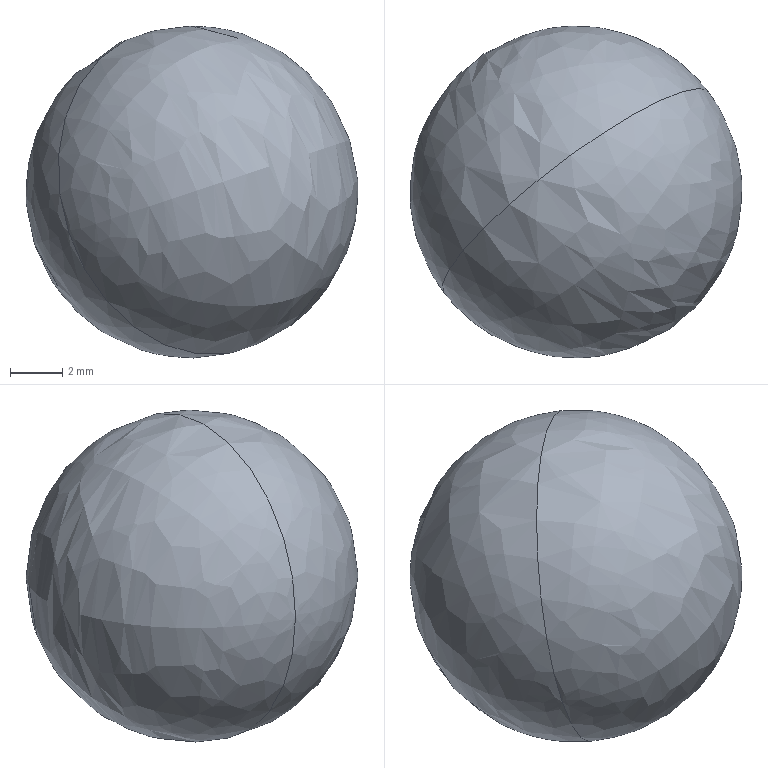Part | SolidWorks | features BaseBody 1 | 1 solid | 2 faces | box 12.7 x 12.7 x 12.7 mm | volume 1073 mm3 | spline 2
STEP:
#1=CARTESIAN_POINT('',(4.713,78.959,80.763));
#2=VERTEX_POINT('',#1);
#3=CARTESIAN_POINT('',(-4.713,71.041,77.637));
#4=VERTEX_POINT('',#3);
#5=CARTESIAN_POINT('',(0.,75.,79.2));
#6=DIRECTION('',(0.592,-0.7819,0.1954));
#7=DIRECTION('',(0.7421,0.6234,0.2461));
#8=AXIS2_PLACEMENT_3D('',#5,#6,#7);
#9=CIRCLE('',#8,6.35);
#10=EDGE_CURVE('',#2,#4,#9,.T.);
#11=ORIENTED_EDGE('',*,*,#10,.F.);
#12=CARTESIAN_POINT('',(0.,75.,79.2));
#13=DIRECTION('',(-0.592,0.7819,-0.1954));
#14=DIRECTION('',(0.7421,0.6234,0.2461));
#15=AXIS2_PLACEMENT_3D('',#12,#13,#14);
#16=CIRCLE('',#15,6.35);
#17=EDGE_CURVE('',#2,#4,#16,.T.);
#18=ORIENTED_EDGE('',*,*,#17,.T.);
#19=EDGE_LOOP('',(#11,#18));
#20=FACE_OUTER_BOUND('',#19,.T.);
#21=CARTESIAN_POINT('',(4.713,78.959,80.763));
#22=CARTESIAN_POINT('',(4.713,78.959,80.763));
#23=CARTESIAN_POINT('',(4.713,78.959,80.763));
#24=CARTESIAN_POINT('',(4.713,78.959,80.763));
#25=CARTESIAN_POINT('',(8.703,78.968,68.706));
#26=CARTESIAN_POINT('',(-6.334,98.828,63.744));
#27=CARTESIAN_POINT('',(-14.316,98.809,87.857));
#28=CARTESIAN_POINT('',(0.7218,78.95,92.82));
#29=CARTESIAN_POINT('',(-0.7218,71.05,65.58));
#30=CARTESIAN_POINT('',(-15.759,90.91,60.618));
#31=CARTESIAN_POINT('',(-23.741,90.892,84.731));
#32=CARTESIAN_POINT('',(-8.703,71.032,89.694));
#33=CARTESIAN_POINT('',(-4.713,71.041,77.637));
#34=CARTESIAN_POINT('',(-4.713,71.041,77.637));
#35=CARTESIAN_POINT('',(-4.713,71.041,77.637));
#36=CARTESIAN_POINT('',(-4.713,71.041,77.637));
#37=(BOUNDED_SURFACE()B_SPLINE_SURFACE(3,3,((#21,#22,#23,#24),(#25,#26,#27,#28),(#29,#30,#31,#32),(#33,#34,#35,#36)),.UNSPECIFIED.,.F.,.F.,.F.)B_SPLINE_SURFACE_WITH_KNOTS((4,4),(4,4),(0.,1.),(0.,1.),.UNSPECIFIED.)GEOMETRIC_REPRESENTATION_ITEM()RATIONAL_B_SPLINE_SURFACE(((1.,0.3333,0.3333,1.),(0.3333,0.1111,0.1111,0.3333),(0.3333,0.1111,0.1111,0.3333),(1.,0.3333,0.3333,1.)))REPRESENTATION_ITEM('')SURFACE());
#38=ADVANCED_FACE('',(#20),#37,.T.);
#39=ORIENTED_EDGE('',*,*,#17,.F.);
#40=ORIENTED_EDGE('',*,*,#10,.T.);
#41=EDGE_LOOP('',(#39,#40));
#42=FACE_OUTER_BOUND('',#41,.T.);
#43=CARTESIAN_POINT('',(4.713,78.959,80.763));
#44=CARTESIAN_POINT('',(4.713,78.959,80.763));
#45=CARTESIAN_POINT('',(4.713,78.959,80.763));
#46=CARTESIAN_POINT('',(4.713,78.959,80.763));
#47=CARTESIAN_POINT('',(0.7218,78.95,92.82));
#48=CARTESIAN_POINT('',(15.759,59.09,97.782));
#49=CARTESIAN_POINT('',(23.741,59.108,73.669));
#50=CARTESIAN_POINT('',(8.703,78.968,68.706));
#51=CARTESIAN_POINT('',(-8.703,71.032,89.694));
#52=CARTESIAN_POINT('',(6.334,51.172,94.656));
#53=CARTESIAN_POINT('',(14.316,51.191,70.543));
#54=CARTESIAN_POINT('',(-0.7218,71.05,65.58));
#55=CARTESIAN_POINT('',(-4.713,71.041,77.637));
#56=CARTESIAN_POINT('',(-4.713,71.041,77.637));
#57=CARTESIAN_POINT('',(-4.713,71.041,77.637));
#58=CARTESIAN_POINT('',(-4.713,71.041,77.637));
#59=(BOUNDED_SURFACE()B_SPLINE_SURFACE(3,3,((#43,#44,#45,#46),(#47,#48,#49,#50),(#51,#52,#53,#54),(#55,#56,#57,#58)),.UNSPECIFIED.,.F.,.F.,.F.)B_SPLINE_SURFACE_WITH_KNOTS((4,4),(4,4),(0.,1.),(0.,1.),.UNSPECIFIED.)GEOMETRIC_REPRESENTATION_ITEM()RATIONAL_B_SPLINE_SURFACE(((1.,0.3333,0.3333,1.),(0.3333,0.1111,0.1111,0.3333),(0.3333,0.1111,0.1111,0.3333),(1.,0.3333,0.3333,1.)))REPRESENTATION_ITEM('')SURFACE());
#60=ADVANCED_FACE('',(#42),#59,.T.);
#61=CLOSED_SHELL('',(#38,#60));
#62=MANIFOLD_SOLID_BREP('',#61);
#63=CARTESIAN_POINT('',(0.,0.,0.));
#64=DIRECTION('',(0.,0.,1.));
#65=DIRECTION('',(1.,0.,0.));
#66=AXIS2_PLACEMENT_3D('',#63,#64,#65);
#67=(LENGTH_UNIT()NAMED_UNIT(*)SI_UNIT(.MILLI.,.METRE.));
#68=UNCERTAINTY_MEASURE_WITH_UNIT(LENGTH_MEASURE(0.00001),#67,'','');
#69=(NAMED_UNIT(*)PLANE_ANGLE_UNIT()SI_UNIT($,.RADIAN.));
#70=(NAMED_UNIT(*)SI_UNIT($,.STERADIAN.)SOLID_ANGLE_UNIT());
#71=(GEOMETRIC_REPRESENTATION_CONTEXT(3)GLOBAL_UNCERTAINTY_ASSIGNED_CONTEXT((#68))GLOBAL_UNIT_ASSIGNED_CONTEXT((#67,#69,#70))REPRESENTATION_CONTEXT('',''));
#72=ADVANCED_BREP_SHAPE_REPRESENTATION('',(#62,#66),#71);